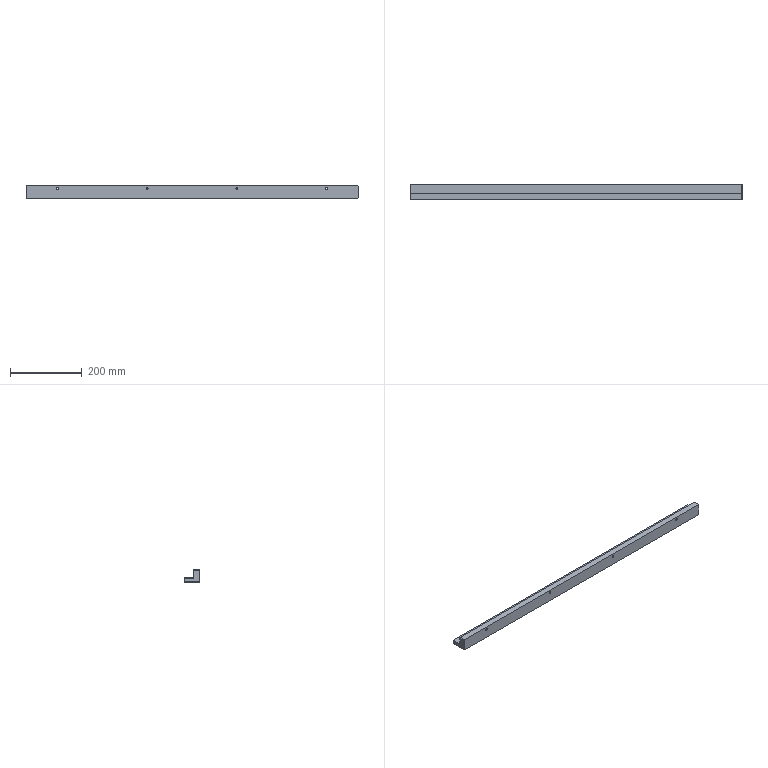Part | NX | features BREP 1 | 1 solid | 54 faces | box 926 x 44 x 35 mm | volume 847450 mm3 | cylinder 26 | plane 18 | cone 10 | commonest cylinder face diameters 3.3 x10 5.5 x8 10 x8
STEP:
#1=CARTESIAN_POINT('',(-463.,17.,16.5));
#2=VERTEX_POINT('',#1);
#3=CARTESIAN_POINT('',(-462.,17.,17.5));
#4=VERTEX_POINT('',#3);
#5=CARTESIAN_POINT('',(-462.,17.,17.5));
#6=DIRECTION('',(0.7071,0.,0.7071));
#7=VECTOR('',#6,1000.);
#8=LINE('',#5,#7);
#9=EDGE_CURVE('',#2,#4,#8,.T.);
#10=ORIENTED_EDGE('',*,*,#9,.F.);
#11=CARTESIAN_POINT('',(-463.,0.,16.5));
#12=VERTEX_POINT('',#11);
#13=CARTESIAN_POINT('',(-463.,44.,16.5));
#14=DIRECTION('',(0.,1.,0.));
#15=VECTOR('',#14,1000.);
#16=LINE('',#13,#15);
#17=EDGE_CURVE('',#12,#2,#16,.T.);
#18=ORIENTED_EDGE('',*,*,#17,.F.);
#19=CARTESIAN_POINT('',(-462.,0.,17.5));
#20=VERTEX_POINT('',#19);
#21=CARTESIAN_POINT('',(-462.,0.,17.5));
#22=DIRECTION('',(-0.7071,0.,-0.7071));
#23=VECTOR('',#22,1000.);
#24=LINE('',#21,#23);
#25=EDGE_CURVE('',#20,#12,#24,.T.);
#26=ORIENTED_EDGE('',*,*,#25,.F.);
#27=CARTESIAN_POINT('',(-462.,44.,17.5));
#28=DIRECTION('',(0.,-1.,0.));
#29=VECTOR('',#28,1000.);
#30=LINE('',#27,#29);
#31=EDGE_CURVE('',#4,#20,#30,.T.);
#32=ORIENTED_EDGE('',*,*,#31,.F.);
#33=EDGE_LOOP('',(#10,#18,#26,#32));
#34=FACE_BOUND('',#33,.T.);
#35=CARTESIAN_POINT('',(-462.,44.,17.5));
#36=DIRECTION('',(0.7071,0.,-0.7071));
#37=DIRECTION('',(0.,-1.,0.));
#38=AXIS2_PLACEMENT_3D('',#35,#36,#37);
#39=PLANE('',#38);
#40=ADVANCED_FACE('',(#34),#39,.F.);
#41=CARTESIAN_POINT('',(-463.,44.,-6.5));
#42=VERTEX_POINT('',#41);
#43=CARTESIAN_POINT('',(-462.,44.,-5.5));
#44=VERTEX_POINT('',#43);
#45=CARTESIAN_POINT('',(-228.25,44.,228.25));
#46=DIRECTION('',(0.7071,0.,0.7071));
#47=VECTOR('',#46,1000.);
#48=LINE('',#45,#47);
#49=EDGE_CURVE('',#42,#44,#48,.T.);
#50=ORIENTED_EDGE('',*,*,#49,.F.);
#51=CARTESIAN_POINT('',(-463.,17.,-6.5));
#52=VERTEX_POINT('',#51);
#53=CARTESIAN_POINT('',(-463.,44.,-6.5));
#54=DIRECTION('',(0.,1.,0.));
#55=VECTOR('',#54,1000.);
#56=LINE('',#53,#55);
#57=EDGE_CURVE('',#52,#42,#56,.T.);
#58=ORIENTED_EDGE('',*,*,#57,.F.);
#59=CARTESIAN_POINT('',(-462.,17.,-5.5));
#60=VERTEX_POINT('',#59);
#61=CARTESIAN_POINT('',(12.,17.,468.5));
#62=DIRECTION('',(-0.7071,0.,-0.7071));
#63=VECTOR('',#62,1000.);
#64=LINE('',#61,#63);
#65=EDGE_CURVE('',#60,#52,#64,.T.);
#66=ORIENTED_EDGE('',*,*,#65,.F.);
#67=CARTESIAN_POINT('',(-462.,44.,-5.5));
#68=DIRECTION('',(0.,-1.,0.));
#69=VECTOR('',#68,1000.);
#70=LINE('',#67,#69);
#71=EDGE_CURVE('',#44,#60,#70,.T.);
#72=ORIENTED_EDGE('',*,*,#71,.F.);
#73=EDGE_LOOP('',(#50,#58,#66,#72));
#74=FACE_BOUND('',#73,.T.);
#75=CARTESIAN_POINT('',(-462.,44.,-5.5));
#76=DIRECTION('',(0.7071,0.,-0.7071));
#77=DIRECTION('',(0.,-1.,0.));
#78=AXIS2_PLACEMENT_3D('',#75,#76,#77);
#79=PLANE('',#78);
#80=ADVANCED_FACE('',(#74),#79,.F.);
#81=CARTESIAN_POINT('',(-462.,44.,-17.5));
#82=VERTEX_POINT('',#81);
#83=CARTESIAN_POINT('',(-463.,44.,-16.5));
#84=VERTEX_POINT('',#83);
#85=CARTESIAN_POINT('',(-239.75,44.,-239.75));
#86=DIRECTION('',(-0.7071,0.,0.7071));
#87=VECTOR('',#86,1000.);
#88=LINE('',#85,#87);
#89=EDGE_CURVE('',#82,#84,#88,.T.);
#90=ORIENTED_EDGE('',*,*,#89,.F.);
#91=CARTESIAN_POINT('',(-462.,0.,-17.5));
#92=VERTEX_POINT('',#91);
#93=CARTESIAN_POINT('',(-462.,44.,-17.5));
#94=DIRECTION('',(0.,1.,0.));
#95=VECTOR('',#94,1000.);
#96=LINE('',#93,#95);
#97=EDGE_CURVE('',#92,#82,#96,.T.);
#98=ORIENTED_EDGE('',*,*,#97,.F.);
#99=CARTESIAN_POINT('',(-463.,0.,-16.5));
#100=VERTEX_POINT('',#99);
#101=CARTESIAN_POINT('',(-463.,0.,-16.5));
#102=DIRECTION('',(0.7071,0.,-0.7071));
#103=VECTOR('',#102,1000.);
#104=LINE('',#101,#103);
#105=EDGE_CURVE('',#100,#92,#104,.T.);
#106=ORIENTED_EDGE('',*,*,#105,.F.);
#107=CARTESIAN_POINT('',(-463.,44.,-16.5));
#108=DIRECTION('',(0.,-1.,0.));
#109=VECTOR('',#108,1000.);
#110=LINE('',#107,#109);
#111=EDGE_CURVE('',#84,#100,#110,.T.);
#112=ORIENTED_EDGE('',*,*,#111,.F.);
#113=EDGE_LOOP('',(#90,#98,#106,#112));
#114=FACE_BOUND('',#113,.T.);
#115=CARTESIAN_POINT('',(-463.,44.,-16.5));
#116=DIRECTION('',(0.7071,0.,0.7071));
#117=DIRECTION('',(0.,-1.,0.));
#118=AXIS2_PLACEMENT_3D('',#115,#116,#117);
#119=PLANE('',#118);
#120=ADVANCED_FACE('',(#114),#119,.F.);
#121=CARTESIAN_POINT('',(462.,44.,-5.5));
#122=VERTEX_POINT('',#121);
#123=CARTESIAN_POINT('',(463.,44.,-6.5));
#124=VERTEX_POINT('',#123);
#125=CARTESIAN_POINT('',(228.25,44.,228.25));
#126=DIRECTION('',(0.7071,0.,-0.7071));
#127=VECTOR('',#126,1000.);
#128=LINE('',#125,#127);
#129=EDGE_CURVE('',#122,#124,#128,.T.);
#130=ORIENTED_EDGE('',*,*,#129,.F.);
#131=CARTESIAN_POINT('',(462.,17.,-5.5));
#132=VERTEX_POINT('',#131);
#133=CARTESIAN_POINT('',(462.,44.,-5.5));
#134=DIRECTION('',(0.,1.,0.));
#135=VECTOR('',#134,1000.);
#136=LINE('',#133,#135);
#137=EDGE_CURVE('',#132,#122,#136,.T.);
#138=ORIENTED_EDGE('',*,*,#137,.F.);
#139=CARTESIAN_POINT('',(463.,17.,-6.5));
#140=VERTEX_POINT('',#139);
#141=CARTESIAN_POINT('',(451.,17.,5.5));
#142=DIRECTION('',(-0.7071,0.,0.7071));
#143=VECTOR('',#142,1000.);
#144=LINE('',#141,#143);
#145=EDGE_CURVE('',#140,#132,#144,.T.);
#146=ORIENTED_EDGE('',*,*,#145,.F.);
#147=CARTESIAN_POINT('',(463.,44.,-6.5));
#148=DIRECTION('',(0.,-1.,0.));
#149=VECTOR('',#148,1000.);
#150=LINE('',#147,#149);
#151=EDGE_CURVE('',#124,#140,#150,.T.);
#152=ORIENTED_EDGE('',*,*,#151,.F.);
#153=EDGE_LOOP('',(#130,#138,#146,#152));
#154=FACE_BOUND('',#153,.T.);
#155=CARTESIAN_POINT('',(463.,44.,-6.5));
#156=DIRECTION('',(-0.7071,0.,-0.7071));
#157=DIRECTION('',(0.,-1.,0.));
#158=AXIS2_PLACEMENT_3D('',#155,#156,#157);
#159=PLANE('',#158);
#160=ADVANCED_FACE('',(#154),#159,.F.);
#161=CARTESIAN_POINT('',(463.,44.,-16.5));
#162=VERTEX_POINT('',#161);
#163=CARTESIAN_POINT('',(462.,44.,-17.5));
#164=VERTEX_POINT('',#163);
#165=CARTESIAN_POINT('',(239.75,44.,-239.75));
#166=DIRECTION('',(-0.7071,0.,-0.7071));
#167=VECTOR('',#166,1000.);
#168=LINE('',#165,#167);
#169=EDGE_CURVE('',#162,#164,#168,.T.);
#170=ORIENTED_EDGE('',*,*,#169,.F.);
#171=CARTESIAN_POINT('',(463.,0.,-16.5));
#172=VERTEX_POINT('',#171);
#173=CARTESIAN_POINT('',(463.,44.,-16.5));
#174=DIRECTION('',(0.,1.,0.));
#175=VECTOR('',#174,1000.);
#176=LINE('',#173,#175);
#177=EDGE_CURVE('',#172,#162,#176,.T.);
#178=ORIENTED_EDGE('',*,*,#177,.F.);
#179=CARTESIAN_POINT('',(462.,0.,-17.5));
#180=VERTEX_POINT('',#179);
#181=CARTESIAN_POINT('',(462.,0.,-17.5));
#182=DIRECTION('',(0.7071,0.,0.7071));
#183=VECTOR('',#182,1000.);
#184=LINE('',#181,#183);
#185=EDGE_CURVE('',#180,#172,#184,.T.);
#186=ORIENTED_EDGE('',*,*,#185,.F.);
#187=CARTESIAN_POINT('',(462.,44.,-17.5));
#188=DIRECTION('',(0.,-1.,0.));
#189=VECTOR('',#188,1000.);
#190=LINE('',#187,#189);
#191=EDGE_CURVE('',#164,#180,#190,.T.);
#192=ORIENTED_EDGE('',*,*,#191,.F.);
#193=EDGE_LOOP('',(#170,#178,#186,#192));
#194=FACE_BOUND('',#193,.T.);
#195=CARTESIAN_POINT('',(462.,44.,-17.5));
#196=DIRECTION('',(-0.7071,0.,0.7071));
#197=DIRECTION('',(0.,-1.,0.));
#198=AXIS2_PLACEMENT_3D('',#195,#196,#197);
#199=PLANE('',#198);
#200=ADVANCED_FACE('',(#194),#199,.F.);
#201=CARTESIAN_POINT('',(462.,17.,17.5));
#202=VERTEX_POINT('',#201);
#203=CARTESIAN_POINT('',(463.,17.,16.5));
#204=VERTEX_POINT('',#203);
#205=CARTESIAN_POINT('',(463.,17.,16.5));
#206=DIRECTION('',(0.7071,0.,-0.7071));
#207=VECTOR('',#206,1000.);
#208=LINE('',#205,#207);
#209=EDGE_CURVE('',#202,#204,#208,.T.);
#210=ORIENTED_EDGE('',*,*,#209,.F.);
#211=CARTESIAN_POINT('',(462.,0.,17.5));
#212=VERTEX_POINT('',#211);
#213=CARTESIAN_POINT('',(462.,44.,17.5));
#214=DIRECTION('',(0.,1.,0.));
#215=VECTOR('',#214,1000.);
#216=LINE('',#213,#215);
#217=EDGE_CURVE('',#212,#202,#216,.T.);
#218=ORIENTED_EDGE('',*,*,#217,.F.);
#219=CARTESIAN_POINT('',(463.,0.,16.5));
#220=VERTEX_POINT('',#219);
#221=CARTESIAN_POINT('',(463.,0.,16.5));
#222=DIRECTION('',(-0.7071,0.,0.7071));
#223=VECTOR('',#222,1000.);
#224=LINE('',#221,#223);
#225=EDGE_CURVE('',#220,#212,#224,.T.);
#226=ORIENTED_EDGE('',*,*,#225,.F.);
#227=CARTESIAN_POINT('',(463.,44.,16.5));
#228=DIRECTION('',(0.,-1.,0.));
#229=VECTOR('',#228,1000.);
#230=LINE('',#227,#229);
#231=EDGE_CURVE('',#204,#220,#230,.T.);
#232=ORIENTED_EDGE('',*,*,#231,.F.);
#233=EDGE_LOOP('',(#210,#218,#226,#232));
#234=FACE_BOUND('',#233,.T.);
#235=CARTESIAN_POINT('',(463.,44.,16.5));
#236=DIRECTION('',(-0.7071,0.,-0.7071));
#237=DIRECTION('',(0.,-1.,0.));
#238=AXIS2_PLACEMENT_3D('',#235,#236,#237);
#239=PLANE('',#238);
#240=ADVANCED_FACE('',(#234),#239,.F.);
#241=CARTESIAN_POINT('',(-375.,17.,4.5));
#242=VERTEX_POINT('',#241);
#243=CARTESIAN_POINT('',(-375.,11.3,4.5));
#244=VERTEX_POINT('',#243);
#245=CARTESIAN_POINT('',(-375.,17.,4.5));
#246=DIRECTION('',(0.,1.,0.));
#247=VECTOR('',#246,1000.);
#248=LINE('',#245,#247);
#249=EDGE_CURVE('',#242,#244,#248,.F.);
#250=ORIENTED_EDGE('',*,*,#249,.T.);
#251=CARTESIAN_POINT('',(-375.,11.3,14.5));
#252=VERTEX_POINT('',#251);
#253=CARTESIAN_POINT('',(-375.,11.3,9.5));
#254=DIRECTION('',(0.,1.,0.));
#255=DIRECTION('',(0.,0.,1.));
#256=AXIS2_PLACEMENT_3D('',#253,#254,#255);
#257=CIRCLE('',#256,5.);
#258=EDGE_CURVE('',#252,#244,#257,.T.);
#259=ORIENTED_EDGE('',*,*,#258,.F.);
#260=CARTESIAN_POINT('',(-375.,17.,14.5));
#261=VERTEX_POINT('',#260);
#262=CARTESIAN_POINT('',(-375.,17.,14.5));
#263=DIRECTION('',(0.,1.,0.));
#264=VECTOR('',#263,1000.);
#265=LINE('',#262,#264);
#266=EDGE_CURVE('',#261,#252,#265,.F.);
#267=ORIENTED_EDGE('',*,*,#266,.F.);
#268=CARTESIAN_POINT('',(-375.,17.,9.5));
#269=DIRECTION('',(0.,1.,0.));
#270=DIRECTION('',(0.,0.,1.));
#271=AXIS2_PLACEMENT_3D('',#268,#269,#270);
#272=CIRCLE('',#271,5.);
#273=EDGE_CURVE('',#261,#242,#272,.T.);
#274=ORIENTED_EDGE('',*,*,#273,.T.);
#275=EDGE_LOOP('',(#250,#259,#267,#274));
#276=FACE_BOUND('',#275,.T.);
#277=CARTESIAN_POINT('',(-375.,17.,9.5));
#278=DIRECTION('',(0.,1.,0.));
#279=DIRECTION('',(0.,0.,1.));
#280=AXIS2_PLACEMENT_3D('',#277,#278,#279);
#281=CYLINDRICAL_SURFACE('',#280,5.);
#282=ADVANCED_FACE('',(#276),#281,.F.);
#283=ORIENTED_EDGE('',*,*,#258,.T.);
#284=CARTESIAN_POINT('',(-375.,11.3,9.5));
#285=DIRECTION('',(0.,1.,0.));
#286=DIRECTION('',(0.,0.,1.));
#287=AXIS2_PLACEMENT_3D('',#284,#285,#286);
#288=CIRCLE('',#287,5.);
#289=EDGE_CURVE('',#244,#252,#288,.T.);
#290=ORIENTED_EDGE('',*,*,#289,.T.);
#291=EDGE_LOOP('',(#283,#290));
#292=FACE_BOUND('',#291,.T.);
#293=CARTESIAN_POINT('',(-375.,11.3,12.25));
#294=VERTEX_POINT('',#293);
#295=CARTESIAN_POINT('',(-375.,11.3,6.75));
#296=VERTEX_POINT('',#295);
#297=CARTESIAN_POINT('',(-375.,11.3,9.5));
#298=DIRECTION('',(0.,1.,0.));
#299=DIRECTION('',(0.,0.,1.));
#300=AXIS2_PLACEMENT_3D('',#297,#298,#299);
#301=CIRCLE('',#300,2.75);
#302=EDGE_CURVE('',#294,#296,#301,.T.);
#303=ORIENTED_EDGE('',*,*,#302,.F.);
#304=CARTESIAN_POINT('',(-375.,11.3,9.5));
#305=DIRECTION('',(0.,1.,0.));
#306=DIRECTION('',(0.,0.,1.));
#307=AXIS2_PLACEMENT_3D('',#304,#305,#306);
#308=CIRCLE('',#307,2.75);
#309=EDGE_CURVE('',#296,#294,#308,.T.);
#310=ORIENTED_EDGE('',*,*,#309,.F.);
#311=EDGE_LOOP('',(#303,#310));
#312=FACE_BOUND('',#311,.T.);
#313=CARTESIAN_POINT('',(-372.25,11.3,9.5));
#314=DIRECTION('',(0.,-1.,0.));
#315=DIRECTION('',(0.,0.,-1.));
#316=AXIS2_PLACEMENT_3D('',#313,#314,#315);
#317=PLANE('',#316);
#318=ADVANCED_FACE('',(#292,#312),#317,.F.);
#319=CARTESIAN_POINT('',(-375.,0.,6.75));
#320=VERTEX_POINT('',#319);
#321=CARTESIAN_POINT('',(-375.,17.,6.75));
#322=DIRECTION('',(0.,1.,0.));
#323=VECTOR('',#322,1000.);
#324=LINE('',#321,#323);
#325=EDGE_CURVE('',#296,#320,#324,.F.);
#326=ORIENTED_EDGE('',*,*,#325,.T.);
#327=CARTESIAN_POINT('',(-375.,0.,12.25));
#328=VERTEX_POINT('',#327);
#329=CARTESIAN_POINT('',(-375.,0.,9.5));
#330=DIRECTION('',(0.,1.,0.));
#331=DIRECTION('',(0.,0.,1.));
#332=AXIS2_PLACEMENT_3D('',#329,#330,#331);
#333=CIRCLE('',#332,2.75);
#334=EDGE_CURVE('',#328,#320,#333,.T.);
#335=ORIENTED_EDGE('',*,*,#334,.F.);
#336=CARTESIAN_POINT('',(-375.,17.,12.25));
#337=DIRECTION('',(0.,1.,0.));
#338=VECTOR('',#337,1000.);
#339=LINE('',#336,#338);
#340=EDGE_CURVE('',#294,#328,#339,.F.);
#341=ORIENTED_EDGE('',*,*,#340,.F.);
#342=ORIENTED_EDGE('',*,*,#302,.T.);
#343=EDGE_LOOP('',(#326,#335,#341,#342));
#344=FACE_BOUND('',#343,.T.);
#345=CARTESIAN_POINT('',(-375.,17.,9.5));
#346=DIRECTION('',(0.,1.,0.));
#347=DIRECTION('',(0.,0.,1.));
#348=AXIS2_PLACEMENT_3D('',#345,#346,#347);
#349=CYLINDRICAL_SURFACE('',#348,2.75);
#350=ADVANCED_FACE('',(#344),#349,.F.);
#351=CARTESIAN_POINT('',(-125.,17.,4.5));
#352=VERTEX_POINT('',#351);
#353=CARTESIAN_POINT('',(-125.,11.3,4.5));
#354=VERTEX_POINT('',#353);
#355=CARTESIAN_POINT('',(-125.,17.,4.5));
#356=DIRECTION('',(0.,1.,0.));
#357=VECTOR('',#356,1000.);
#358=LINE('',#355,#357);
#359=EDGE_CURVE('',#352,#354,#358,.F.);
#360=ORIENTED_EDGE('',*,*,#359,.T.);
#361=CARTESIAN_POINT('',(-125.,11.3,14.5));
#362=VERTEX_POINT('',#361);
#363=CARTESIAN_POINT('',(-125.,11.3,9.5));
#364=DIRECTION('',(0.,1.,0.));
#365=DIRECTION('',(0.,0.,1.));
#366=AXIS2_PLACEMENT_3D('',#363,#364,#365);
#367=CIRCLE('',#366,5.);
#368=EDGE_CURVE('',#362,#354,#367,.T.);
#369=ORIENTED_EDGE('',*,*,#368,.F.);
#370=CARTESIAN_POINT('',(-125.,17.,14.5));
#371=VERTEX_POINT('',#370);
#372=CARTESIAN_POINT('',(-125.,17.,14.5));
#373=DIRECTION('',(0.,1.,0.));
#374=VECTOR('',#373,1000.);
#375=LINE('',#372,#374);
#376=EDGE_CURVE('',#371,#362,#375,.F.);
#377=ORIENTED_EDGE('',*,*,#376,.F.);
#378=CARTESIAN_POINT('',(-125.,17.,9.5));
#379=DIRECTION('',(0.,1.,0.));
#380=DIRECTION('',(0.,0.,1.));
#381=AXIS2_PLACEMENT_3D('',#378,#379,#380);
#382=CIRCLE('',#381,5.);
#383=EDGE_CURVE('',#371,#352,#382,.T.);
#384=ORIENTED_EDGE('',*,*,#383,.T.);
#385=EDGE_LOOP('',(#360,#369,#377,#384));
#386=FACE_BOUND('',#385,.T.);
#387=CARTESIAN_POINT('',(-125.,17.,9.5));
#388=DIRECTION('',(0.,1.,0.));
#389=DIRECTION('',(0.,0.,1.));
#390=AXIS2_PLACEMENT_3D('',#387,#388,#389);
#391=CYLINDRICAL_SURFACE('',#390,5.);
#392=ADVANCED_FACE('',(#386),#391,.F.);
#393=ORIENTED_EDGE('',*,*,#368,.T.);
#394=CARTESIAN_POINT('',(-125.,11.3,9.5));
#395=DIRECTION('',(0.,1.,0.));
#396=DIRECTION('',(0.,0.,1.));
#397=AXIS2_PLACEMENT_3D('',#394,#395,#396);
#398=CIRCLE('',#397,5.);
#399=EDGE_CURVE('',#354,#362,#398,.T.);
#400=ORIENTED_EDGE('',*,*,#399,.T.);
#401=EDGE_LOOP('',(#393,#400));
#402=FACE_BOUND('',#401,.T.);
#403=CARTESIAN_POINT('',(-125.,11.3,12.25));
#404=VERTEX_POINT('',#403);
#405=CARTESIAN_POINT('',(-125.,11.3,6.75));
#406=VERTEX_POINT('',#405);
#407=CARTESIAN_POINT('',(-125.,11.3,9.5));
#408=DIRECTION('',(0.,1.,0.));
#409=DIRECTION('',(0.,0.,1.));
#410=AXIS2_PLACEMENT_3D('',#407,#408,#409);
#411=CIRCLE('',#410,2.75);
#412=EDGE_CURVE('',#404,#406,#411,.T.);
#413=ORIENTED_EDGE('',*,*,#412,.F.);
#414=CARTESIAN_POINT('',(-125.,11.3,9.5));
#415=DIRECTION('',(0.,1.,0.));
#416=DIRECTION('',(0.,0.,1.));
#417=AXIS2_PLACEMENT_3D('',#414,#415,#416);
#418=CIRCLE('',#417,2.75);
#419=EDGE_CURVE('',#406,#404,#418,.T.);
#420=ORIENTED_EDGE('',*,*,#419,.F.);
#421=EDGE_LOOP('',(#413,#420));
#422=FACE_BOUND('',#421,.T.);
#423=CARTESIAN_POINT('',(-122.25,11.3,9.5));
#424=DIRECTION('',(0.,-1.,0.));
#425=DIRECTION('',(0.,0.,-1.));
#426=AXIS2_PLACEMENT_3D('',#423,#424,#425);
#427=PLANE('',#426);
#428=ADVANCED_FACE('',(#402,#422),#427,.F.);
#429=CARTESIAN_POINT('',(-125.,0.,6.75));
#430=VERTEX_POINT('',#429);
#431=CARTESIAN_POINT('',(-125.,17.,6.75));
#432=DIRECTION('',(0.,1.,0.));
#433=VECTOR('',#432,1000.);
#434=LINE('',#431,#433);
#435=EDGE_CURVE('',#406,#430,#434,.F.);
#436=ORIENTED_EDGE('',*,*,#435,.T.);
#437=CARTESIAN_POINT('',(-125.,0.,12.25));
#438=VERTEX_POINT('',#437);
#439=CARTESIAN_POINT('',(-125.,0.,9.5));
#440=DIRECTION('',(0.,1.,0.));
#441=DIRECTION('',(0.,0.,1.));
#442=AXIS2_PLACEMENT_3D('',#439,#440,#441);
#443=CIRCLE('',#442,2.75);
#444=EDGE_CURVE('',#438,#430,#443,.T.);
#445=ORIENTED_EDGE('',*,*,#444,.F.);
#446=CARTESIAN_POINT('',(-125.,17.,12.25));
#447=DIRECTION('',(0.,1.,0.));
#448=VECTOR('',#447,1000.);
#449=LINE('',#446,#448);
#450=EDGE_CURVE('',#404,#438,#449,.F.);
#451=ORIENTED_EDGE('',*,*,#450,.F.);
#452=ORIENTED_EDGE('',*,*,#412,.T.);
#453=EDGE_LOOP('',(#436,#445,#451,#452));
#454=FACE_BOUND('',#453,.T.);
#455=CARTESIAN_POINT('',(-125.,17.,9.5));
#456=DIRECTION('',(0.,1.,0.));
#457=DIRECTION('',(0.,0.,1.));
#458=AXIS2_PLACEMENT_3D('',#455,#456,#457);
#459=CYLINDRICAL_SURFACE('',#458,2.75);
#460=ADVANCED_FACE('',(#454),#459,.F.);
#461=CARTESIAN_POINT('',(125.,17.,4.5));
#462=VERTEX_POINT('',#461);
#463=CARTESIAN_POINT('',(125.,11.3,4.5));
#464=VERTEX_POINT('',#463);
#465=CARTESIAN_POINT('',(125.,17.,4.5));
#466=DIRECTION('',(0.,1.,0.));
#467=VECTOR('',#466,1000.);
#468=LINE('',#465,#467);
#469=EDGE_CURVE('',#462,#464,#468,.F.);
#470=ORIENTED_EDGE('',*,*,#469,.T.);
#471=CARTESIAN_POINT('',(125.,11.3,14.5));
#472=VERTEX_POINT('',#471);
#473=CARTESIAN_POINT('',(125.,11.3,9.5));
#474=DIRECTION('',(0.,1.,0.));
#475=DIRECTION('',(0.,0.,1.));
#476=AXIS2_PLACEMENT_3D('',#473,#474,#475);
#477=CIRCLE('',#476,5.);
#478=EDGE_CURVE('',#472,#464,#477,.T.);
#479=ORIENTED_EDGE('',*,*,#478,.F.);
#480=CARTESIAN_POINT('',(125.,17.,14.5));
#481=VERTEX_POINT('',#480);
#482=CARTESIAN_POINT('',(125.,17.,14.5));
#483=DIRECTION('',(0.,1.,0.));
#484=VECTOR('',#483,1000.);
#485=LINE('',#482,#484);
#486=EDGE_CURVE('',#481,#472,#485,.F.);
#487=ORIENTED_EDGE('',*,*,#486,.F.);
#488=CARTESIAN_POINT('',(125.,17.,9.5));
#489=DIRECTION('',(0.,1.,0.));
#490=DIRECTION('',(0.,0.,1.));
#491=AXIS2_PLACEMENT_3D('',#488,#489,#490);
#492=CIRCLE('',#491,5.);
#493=EDGE_CURVE('',#481,#462,#492,.T.);
#494=ORIENTED_EDGE('',*,*,#493,.T.);
#495=EDGE_LOOP('',(#470,#479,#487,#494));
#496=FACE_BOUND('',#495,.T.);
#497=CARTESIAN_POINT('',(125.,17.,9.5));
#498=DIRECTION('',(0.,1.,0.));
#499=DIRECTION('',(0.,0.,1.));
#500=AXIS2_PLACEMENT_3D('',#497,#498,#499);
#501=CYLINDRICAL_SURFACE('',#500,5.);
#502=ADVANCED_FACE('',(#496),#501,.F.);
#503=ORIENTED_EDGE('',*,*,#478,.T.);
#504=CARTESIAN_POINT('',(125.,11.3,9.5));
#505=DIRECTION('',(0.,1.,0.));
#506=DIRECTION('',(0.,0.,1.));
#507=AXIS2_PLACEMENT_3D('',#504,#505,#506);
#508=CIRCLE('',#507,5.);
#509=EDGE_CURVE('',#464,#472,#508,.T.);
#510=ORIENTED_EDGE('',*,*,#509,.T.);
#511=EDGE_LOOP('',(#503,#510));
#512=FACE_BOUND('',#511,.T.);
#513=CARTESIAN_POINT('',(125.,11.3,12.25));
#514=VERTEX_POINT('',#513);
#515=CARTESIAN_POINT('',(125.,11.3,6.75));
#516=VERTEX_POINT('',#515);
#517=CARTESIAN_POINT('',(125.,11.3,9.5));
#518=DIRECTION('',(0.,1.,0.));
#519=DIRECTION('',(0.,0.,1.));
#520=AXIS2_PLACEMENT_3D('',#517,#518,#519);
#521=CIRCLE('',#520,2.75);
#522=EDGE_CURVE('',#514,#516,#521,.T.);
#523=ORIENTED_EDGE('',*,*,#522,.F.);
#524=CARTESIAN_POINT('',(125.,11.3,9.5));
#525=DIRECTION('',(0.,1.,0.));
#526=DIRECTION('',(0.,0.,1.));
#527=AXIS2_PLACEMENT_3D('',#524,#525,#526);
#528=CIRCLE('',#527,2.75);
#529=EDGE_CURVE('',#516,#514,#528,.T.);
#530=ORIENTED_EDGE('',*,*,#529,.F.);
#531=EDGE_LOOP('',(#523,#530));
#532=FACE_BOUND('',#531,.T.);
#533=CARTESIAN_POINT('',(127.75,11.3,9.5));
#534=DIRECTION('',(0.,-1.,0.));
#535=DIRECTION('',(0.,0.,-1.));
#536=AXIS2_PLACEMENT_3D('',#533,#534,#535);
#537=PLANE('',#536);
#538=ADVANCED_FACE('',(#512,#532),#537,.F.);
#539=CARTESIAN_POINT('',(125.,0.,6.75));
#540=VERTEX_POINT('',#539);
#541=CARTESIAN_POINT('',(125.,17.,6.75));
#542=DIRECTION('',(0.,1.,0.));
#543=VECTOR('',#542,1000.);
#544=LINE('',#541,#543);
#545=EDGE_CURVE('',#516,#540,#544,.F.);
#546=ORIENTED_EDGE('',*,*,#545,.T.);
#547=CARTESIAN_POINT('',(125.,0.,12.25));
#548=VERTEX_POINT('',#547);
#549=CARTESIAN_POINT('',(125.,0.,9.5));
#550=DIRECTION('',(0.,1.,0.));
#551=DIRECTION('',(0.,0.,1.));
#552=AXIS2_PLACEMENT_3D('',#549,#550,#551);
#553=CIRCLE('',#552,2.75);
#554=EDGE_CURVE('',#548,#540,#553,.T.);
#555=ORIENTED_EDGE('',*,*,#554,.F.);
#556=CARTESIAN_POINT('',(125.,17.,12.25));
#557=DIRECTION('',(0.,1.,0.));
#558=VECTOR('',#557,1000.);
#559=LINE('',#556,#558);
#560=EDGE_CURVE('',#514,#548,#559,.F.);
#561=ORIENTED_EDGE('',*,*,#560,.F.);
#562=ORIENTED_EDGE('',*,*,#522,.T.);
#563=EDGE_LOOP('',(#546,#555,#561,#562));
#564=FACE_BOUND('',#563,.T.);
#565=CARTESIAN_POINT('',(125.,17.,9.5));
#566=DIRECTION('',(0.,1.,0.));
#567=DIRECTION('',(0.,0.,1.));
#568=AXIS2_PLACEMENT_3D('',#565,#566,#567);
#569=CYLINDRICAL_SURFACE('',#568,2.75);
#570=ADVANCED_FACE('',(#564),#569,.F.);
#571=CARTESIAN_POINT('',(375.,17.,4.5));
#572=VERTEX_POINT('',#571);
#573=CARTESIAN_POINT('',(375.,11.3,4.5));
#574=VERTEX_POINT('',#573);
#575=CARTESIAN_POINT('',(375.,17.,4.5));
#576=DIRECTION('',(0.,1.,0.));
#577=VECTOR('',#576,1000.);
#578=LINE('',#575,#577);
#579=EDGE_CURVE('',#572,#574,#578,.F.);
#580=ORIENTED_EDGE('',*,*,#579,.T.);
#581=CARTESIAN_POINT('',(375.,11.3,14.5));
#582=VERTEX_POINT('',#581);
#583=CARTESIAN_POINT('',(375.,11.3,9.5));
#584=DIRECTION('',(0.,1.,0.));
#585=DIRECTION('',(0.,0.,1.));
#586=AXIS2_PLACEMENT_3D('',#583,#584,#585);
#587=CIRCLE('',#586,5.);
#588=EDGE_CURVE('',#582,#574,#587,.T.);
#589=ORIENTED_EDGE('',*,*,#588,.F.);
#590=CARTESIAN_POINT('',(375.,17.,14.5));
#591=VERTEX_POINT('',#590);
#592=CARTESIAN_POINT('',(375.,17.,14.5));
#593=DIRECTION('',(0.,1.,0.));
#594=VECTOR('',#593,1000.);
#595=LINE('',#592,#594);
#596=EDGE_CURVE('',#591,#582,#595,.F.);
#597=ORIENTED_EDGE('',*,*,#596,.F.);
#598=CARTESIAN_POINT('',(375.,17.,9.5));
#599=DIRECTION('',(0.,1.,0.));
#600=DIRECTION('',(0.,0.,1.));
#601=AXIS2_PLACEMENT_3D('',#598,#599,#600);
#602=CIRCLE('',#601,5.);
#603=EDGE_CURVE('',#591,#572,#602,.T.);
#604=ORIENTED_EDGE('',*,*,#603,.T.);
#605=EDGE_LOOP('',(#580,#589,#597,#604));
#606=FACE_BOUND('',#605,.T.);
#607=CARTESIAN_POINT('',(375.,17.,9.5));
#608=DIRECTION('',(0.,1.,0.));
#609=DIRECTION('',(0.,0.,1.));
#610=AXIS2_PLACEMENT_3D('',#607,#608,#609);
#611=CYLINDRICAL_SURFACE('',#610,5.);
#612=ADVANCED_FACE('',(#606),#611,.F.);
#613=ORIENTED_EDGE('',*,*,#588,.T.);
#614=CARTESIAN_POINT('',(375.,11.3,9.5));
#615=DIRECTION('',(0.,1.,0.));
#616=DIRECTION('',(0.,0.,1.));
#617=AXIS2_PLACEMENT_3D('',#614,#615,#616);
#618=CIRCLE('',#617,5.);
#619=EDGE_CURVE('',#574,#582,#618,.T.);
#620=ORIENTED_EDGE('',*,*,#619,.T.);
#621=EDGE_LOOP('',(#613,#620));
#622=FACE_BOUND('',#621,.T.);
#623=CARTESIAN_POINT('',(375.,11.3,12.25));
#624=VERTEX_POINT('',#623);
#625=CARTESIAN_POINT('',(375.,11.3,6.75));
#626=VERTEX_POINT('',#625);
#627=CARTESIAN_POINT('',(375.,11.3,9.5));
#628=DIRECTION('',(0.,1.,0.));
#629=DIRECTION('',(0.,0.,1.));
#630=AXIS2_PLACEMENT_3D('',#627,#628,#629);
#631=CIRCLE('',#630,2.75);
#632=EDGE_CURVE('',#624,#626,#631,.T.);
#633=ORIENTED_EDGE('',*,*,#632,.F.);
#634=CARTESIAN_POINT('',(375.,11.3,9.5));
#635=DIRECTION('',(0.,1.,0.));
#636=DIRECTION('',(0.,0.,1.));
#637=AXIS2_PLACEMENT_3D('',#634,#635,#636);
#638=CIRCLE('',#637,2.75);
#639=EDGE_CURVE('',#626,#624,#638,.T.);
#640=ORIENTED_EDGE('',*,*,#639,.F.);
#641=EDGE_LOOP('',(#633,#640));
#642=FACE_BOUND('',#641,.T.);
#643=CARTESIAN_POINT('',(377.75,11.3,9.5));
#644=DIRECTION('',(0.,-1.,0.));
#645=DIRECTION('',(0.,0.,-1.));
#646=AXIS2_PLACEMENT_3D('',#643,#644,#645);
#647=PLANE('',#646);
#648=ADVANCED_FACE('',(#622,#642),#647,.F.);
#649=CARTESIAN_POINT('',(375.,0.,6.75));
#650=VERTEX_POINT('',#649);
#651=CARTESIAN_POINT('',(375.,17.,6.75));
#652=DIRECTION('',(0.,1.,0.));
#653=VECTOR('',#652,1000.);
#654=LINE('',#651,#653);
#655=EDGE_CURVE('',#626,#650,#654,.F.);
#656=ORIENTED_EDGE('',*,*,#655,.T.);
#657=CARTESIAN_POINT('',(375.,0.,12.25));
#658=VERTEX_POINT('',#657);
#659=CARTESIAN_POINT('',(375.,0.,9.5));
#660=DIRECTION('',(0.,1.,0.));
#661=DIRECTION('',(0.,0.,1.));
#662=AXIS2_PLACEMENT_3D('',#659,#660,#661);
#663=CIRCLE('',#662,2.75);
#664=EDGE_CURVE('',#658,#650,#663,.T.);
#665=ORIENTED_EDGE('',*,*,#664,.F.);
#666=CARTESIAN_POINT('',(375.,17.,12.25));
#667=DIRECTION('',(0.,1.,0.));
#668=VECTOR('',#667,1000.);
#669=LINE('',#666,#668);
#670=EDGE_CURVE('',#624,#658,#669,.F.);
#671=ORIENTED_EDGE('',*,*,#670,.F.);
#672=ORIENTED_EDGE('',*,*,#632,.T.);
#673=EDGE_LOOP('',(#656,#665,#671,#672));
#674=FACE_BOUND('',#673,.T.);
#675=CARTESIAN_POINT('',(375.,17.,9.5));
#676=DIRECTION('',(0.,1.,0.));
#677=DIRECTION('',(0.,0.,1.));
#678=AXIS2_PLACEMENT_3D('',#675,#676,#677);
#679=CYLINDRICAL_SURFACE('',#678,2.75);
#680=ADVANCED_FACE('',(#674),#679,.F.);
#681=CARTESIAN_POINT('',(-440.,44.,-13.15));
#682=VERTEX_POINT('',#681);
#683=CARTESIAN_POINT('',(-440.,30.5,-13.15));
#684=VERTEX_POINT('',#683);
#685=CARTESIAN_POINT('',(-440.,44.,-13.15));
#686=DIRECTION('',(0.,1.,0.));
#687=VECTOR('',#686,1000.);
#688=LINE('',#685,#687);
#689=EDGE_CURVE('',#682,#684,#688,.F.);
#690=ORIENTED_EDGE('',*,*,#689,.T.);
#691=CARTESIAN_POINT('',(-440.,30.5,-9.85));
#692=VERTEX_POINT('',#691);
#693=CARTESIAN_POINT('',(-440.,30.5,-11.5));
#694=DIRECTION('',(0.,1.,0.));
#695=DIRECTION('',(0.,0.,1.));
#696=AXIS2_PLACEMENT_3D('',#693,#694,#695);
#697=CIRCLE('',#696,1.65);
#698=EDGE_CURVE('',#692,#684,#697,.T.);
#699=ORIENTED_EDGE('',*,*,#698,.F.);
#700=CARTESIAN_POINT('',(-440.,44.,-9.85));
#701=VERTEX_POINT('',#700);
#702=CARTESIAN_POINT('',(-440.,44.,-9.85));
#703=DIRECTION('',(0.,1.,0.));
#704=VECTOR('',#703,1000.);
#705=LINE('',#702,#704);
#706=EDGE_CURVE('',#701,#692,#705,.F.);
#707=ORIENTED_EDGE('',*,*,#706,.F.);
#708=CARTESIAN_POINT('',(-440.,44.,-11.5));
#709=DIRECTION('',(0.,1.,0.));
#710=DIRECTION('',(0.,0.,1.));
#711=AXIS2_PLACEMENT_3D('',#708,#709,#710);
#712=CIRCLE('',#711,1.65);
#713=EDGE_CURVE('',#701,#682,#712,.T.);
#714=ORIENTED_EDGE('',*,*,#713,.T.);
#715=EDGE_LOOP('',(#690,#699,#707,#714));
#716=FACE_BOUND('',#715,.T.);
#717=CARTESIAN_POINT('',(-440.,44.,-11.5));
#718=DIRECTION('',(0.,1.,0.));
#719=DIRECTION('',(0.,0.,1.));
#720=AXIS2_PLACEMENT_3D('',#717,#718,#719);
#721=CYLINDRICAL_SURFACE('',#720,1.65);
#722=ADVANCED_FACE('',(#716),#721,.F.);
#723=CARTESIAN_POINT('',(-440.,29.509,-11.5));
#724=VERTEX_POINT('',#723);
#725=CARTESIAN_POINT('',(-440.,30.5,-13.15));
#726=DIRECTION('',(0.,0.515,-0.8572));
#727=VECTOR('',#726,1000.);
#728=LINE('',#725,#727);
#729=EDGE_CURVE('',#724,#684,#728,.T.);
#730=ORIENTED_EDGE('',*,*,#729,.F.);
#731=CARTESIAN_POINT('',(-440.,30.5,-9.85));
#732=DIRECTION('',(0.,0.515,0.8572));
#733=VECTOR('',#732,1000.);
#734=LINE('',#731,#733);
#735=EDGE_CURVE('',#724,#692,#734,.T.);
#736=ORIENTED_EDGE('',*,*,#735,.T.);
#737=ORIENTED_EDGE('',*,*,#698,.T.);
#738=EDGE_LOOP('',(#730,#736,#737));
#739=FACE_BOUND('',#738,.T.);
#740=CARTESIAN_POINT('',(-440.,30.5,-11.5));
#741=DIRECTION('',(0.,1.,0.));
#742=DIRECTION('',(0.,0.,1.));
#743=AXIS2_PLACEMENT_3D('',#740,#741,#742);
#744=CONICAL_SURFACE('',#743,1.65,1.03);
#745=ADVANCED_FACE('',(#739),#744,.F.);
#746=CARTESIAN_POINT('',(-220.,44.,-13.15));
#747=VERTEX_POINT('',#746);
#748=CARTESIAN_POINT('',(-220.,30.5,-13.15));
#749=VERTEX_POINT('',#748);
#750=CARTESIAN_POINT('',(-220.,44.,-13.15));
#751=DIRECTION('',(0.,1.,0.));
#752=VECTOR('',#751,1000.);
#753=LINE('',#750,#752);
#754=EDGE_CURVE('',#747,#749,#753,.F.);
#755=ORIENTED_EDGE('',*,*,#754,.T.);
#756=CARTESIAN_POINT('',(-220.,30.5,-9.85));
#757=VERTEX_POINT('',#756);
#758=CARTESIAN_POINT('',(-220.,30.5,-11.5));
#759=DIRECTION('',(0.,1.,0.));
#760=DIRECTION('',(0.,0.,1.));
#761=AXIS2_PLACEMENT_3D('',#758,#759,#760);
#762=CIRCLE('',#761,1.65);
#763=EDGE_CURVE('',#757,#749,#762,.T.);
#764=ORIENTED_EDGE('',*,*,#763,.F.);
#765=CARTESIAN_POINT('',(-220.,44.,-9.85));
#766=VERTEX_POINT('',#765);
#767=CARTESIAN_POINT('',(-220.,44.,-9.85));
#768=DIRECTION('',(0.,1.,0.));
#769=VECTOR('',#768,1000.);
#770=LINE('',#767,#769);
#771=EDGE_CURVE('',#766,#757,#770,.F.);
#772=ORIENTED_EDGE('',*,*,#771,.F.);
#773=CARTESIAN_POINT('',(-220.,44.,-11.5));
#774=DIRECTION('',(0.,1.,0.));
#775=DIRECTION('',(0.,0.,1.));
#776=AXIS2_PLACEMENT_3D('',#773,#774,#775);
#777=CIRCLE('',#776,1.65);
#778=EDGE_CURVE('',#766,#747,#777,.T.);
#779=ORIENTED_EDGE('',*,*,#778,.T.);
#780=EDGE_LOOP('',(#755,#764,#772,#779));
#781=FACE_BOUND('',#780,.T.);
#782=CARTESIAN_POINT('',(-220.,44.,-11.5));
#783=DIRECTION('',(0.,1.,0.));
#784=DIRECTION('',(0.,0.,1.));
#785=AXIS2_PLACEMENT_3D('',#782,#783,#784);
#786=CYLINDRICAL_SURFACE('',#785,1.65);
#787=ADVANCED_FACE('',(#781),#786,.F.);
#788=CARTESIAN_POINT('',(-220.,29.509,-11.5));
#789=VERTEX_POINT('',#788);
#790=CARTESIAN_POINT('',(-220.,30.5,-13.15));
#791=DIRECTION('',(0.,0.515,-0.8572));
#792=VECTOR('',#791,1000.);
#793=LINE('',#790,#792);
#794=EDGE_CURVE('',#789,#749,#793,.T.);
#795=ORIENTED_EDGE('',*,*,#794,.F.);
#796=CARTESIAN_POINT('',(-220.,30.5,-9.85));
#797=DIRECTION('',(0.,0.515,0.8572));
#798=VECTOR('',#797,1000.);
#799=LINE('',#796,#798);
#800=EDGE_CURVE('',#789,#757,#799,.T.);
#801=ORIENTED_EDGE('',*,*,#800,.T.);
#802=ORIENTED_EDGE('',*,*,#763,.T.);
#803=EDGE_LOOP('',(#795,#801,#802));
#804=FACE_BOUND('',#803,.T.);
#805=CARTESIAN_POINT('',(-220.,30.5,-11.5));
#806=DIRECTION('',(0.,1.,0.));
#807=DIRECTION('',(0.,0.,1.));
#808=AXIS2_PLACEMENT_3D('',#805,#806,#807);
#809=CONICAL_SURFACE('',#808,1.65,1.03);
#810=ADVANCED_FACE('',(#804),#809,.F.);
#811=CARTESIAN_POINT('',(0.,44.,-13.15));
#812=VERTEX_POINT('',#811);
#813=CARTESIAN_POINT('',(0.,30.5,-13.15));
#814=VERTEX_POINT('',#813);
#815=CARTESIAN_POINT('',(0.,44.,-13.15));
#816=DIRECTION('',(0.,1.,0.));
#817=VECTOR('',#816,1000.);
#818=LINE('',#815,#817);
#819=EDGE_CURVE('',#812,#814,#818,.F.);
#820=ORIENTED_EDGE('',*,*,#819,.T.);
#821=CARTESIAN_POINT('',(0.,30.5,-9.85));
#822=VERTEX_POINT('',#821);
#823=CARTESIAN_POINT('',(0.,30.5,-11.5));
#824=DIRECTION('',(0.,1.,0.));
#825=DIRECTION('',(0.,0.,1.));
#826=AXIS2_PLACEMENT_3D('',#823,#824,#825);
#827=CIRCLE('',#826,1.65);
#828=EDGE_CURVE('',#822,#814,#827,.T.);
#829=ORIENTED_EDGE('',*,*,#828,.F.);
#830=CARTESIAN_POINT('',(0.,44.,-9.85));
#831=VERTEX_POINT('',#830);
#832=CARTESIAN_POINT('',(0.,44.,-9.85));
#833=DIRECTION('',(0.,1.,0.));
#834=VECTOR('',#833,1000.);
#835=LINE('',#832,#834);
#836=EDGE_CURVE('',#831,#822,#835,.F.);
#837=ORIENTED_EDGE('',*,*,#836,.F.);
#838=CARTESIAN_POINT('',(0.,44.,-11.5));
#839=DIRECTION('',(0.,1.,0.));
#840=DIRECTION('',(0.,0.,1.));
#841=AXIS2_PLACEMENT_3D('',#838,#839,#840);
#842=CIRCLE('',#841,1.65);
#843=EDGE_CURVE('',#831,#812,#842,.T.);
#844=ORIENTED_EDGE('',*,*,#843,.T.);
#845=EDGE_LOOP('',(#820,#829,#837,#844));
#846=FACE_BOUND('',#845,.T.);
#847=CARTESIAN_POINT('',(0.,44.,-11.5));
#848=DIRECTION('',(0.,1.,0.));
#849=DIRECTION('',(0.,0.,1.));
#850=AXIS2_PLACEMENT_3D('',#847,#848,#849);
#851=CYLINDRICAL_SURFACE('',#850,1.65);
#852=ADVANCED_FACE('',(#846),#851,.F.);
#853=CARTESIAN_POINT('',(0.,29.509,-11.5));
#854=VERTEX_POINT('',#853);
#855=CARTESIAN_POINT('',(0.,30.5,-13.15));
#856=DIRECTION('',(0.,0.515,-0.8572));
#857=VECTOR('',#856,1000.);
#858=LINE('',#855,#857);
#859=EDGE_CURVE('',#854,#814,#858,.T.);
#860=ORIENTED_EDGE('',*,*,#859,.F.);
#861=CARTESIAN_POINT('',(0.,30.5,-9.85));
#862=DIRECTION('',(0.,0.515,0.8572));
#863=VECTOR('',#862,1000.);
#864=LINE('',#861,#863);
#865=EDGE_CURVE('',#854,#822,#864,.T.);
#866=ORIENTED_EDGE('',*,*,#865,.T.);
#867=ORIENTED_EDGE('',*,*,#828,.T.);
#868=EDGE_LOOP('',(#860,#866,#867));
#869=FACE_BOUND('',#868,.T.);
#870=CARTESIAN_POINT('',(0.,30.5,-11.5));
#871=DIRECTION('',(0.,1.,0.));
#872=DIRECTION('',(0.,0.,1.));
#873=AXIS2_PLACEMENT_3D('',#870,#871,#872);
#874=CONICAL_SURFACE('',#873,1.65,1.03);
#875=ADVANCED_FACE('',(#869),#874,.F.);
#876=CARTESIAN_POINT('',(220.,44.,-13.15));
#877=VERTEX_POINT('',#876);
#878=CARTESIAN_POINT('',(220.,30.5,-13.15));
#879=VERTEX_POINT('',#878);
#880=CARTESIAN_POINT('',(220.,44.,-13.15));
#881=DIRECTION('',(0.,1.,0.));
#882=VECTOR('',#881,1000.);
#883=LINE('',#880,#882);
#884=EDGE_CURVE('',#877,#879,#883,.F.);
#885=ORIENTED_EDGE('',*,*,#884,.T.);
#886=CARTESIAN_POINT('',(220.,30.5,-9.85));
#887=VERTEX_POINT('',#886);
#888=CARTESIAN_POINT('',(220.,30.5,-11.5));
#889=DIRECTION('',(0.,1.,0.));
#890=DIRECTION('',(0.,0.,1.));
#891=AXIS2_PLACEMENT_3D('',#888,#889,#890);
#892=CIRCLE('',#891,1.65);
#893=EDGE_CURVE('',#887,#879,#892,.T.);
#894=ORIENTED_EDGE('',*,*,#893,.F.);
#895=CARTESIAN_POINT('',(220.,44.,-9.85));
#896=VERTEX_POINT('',#895);
#897=CARTESIAN_POINT('',(220.,44.,-9.85));
#898=DIRECTION('',(0.,1.,0.));
#899=VECTOR('',#898,1000.);
#900=LINE('',#897,#899);
#901=EDGE_CURVE('',#896,#887,#900,.F.);
#902=ORIENTED_EDGE('',*,*,#901,.F.);
#903=CARTESIAN_POINT('',(220.,44.,-11.5));
#904=DIRECTION('',(0.,1.,0.));
#905=DIRECTION('',(0.,0.,1.));
#906=AXIS2_PLACEMENT_3D('',#903,#904,#905);
#907=CIRCLE('',#906,1.65);
#908=EDGE_CURVE('',#896,#877,#907,.T.);
#909=ORIENTED_EDGE('',*,*,#908,.T.);
#910=EDGE_LOOP('',(#885,#894,#902,#909));
#911=FACE_BOUND('',#910,.T.);
#912=CARTESIAN_POINT('',(220.,44.,-11.5));
#913=DIRECTION('',(0.,1.,0.));
#914=DIRECTION('',(0.,0.,1.));
#915=AXIS2_PLACEMENT_3D('',#912,#913,#914);
#916=CYLINDRICAL_SURFACE('',#915,1.65);
#917=ADVANCED_FACE('',(#911),#916,.F.);
#918=CARTESIAN_POINT('',(220.,29.509,-11.5));
#919=VERTEX_POINT('',#918);
#920=CARTESIAN_POINT('',(220.,30.5,-13.15));
#921=DIRECTION('',(0.,0.515,-0.8572));
#922=VECTOR('',#921,1000.);
#923=LINE('',#920,#922);
#924=EDGE_CURVE('',#919,#879,#923,.T.);
#925=ORIENTED_EDGE('',*,*,#924,.F.);
#926=CARTESIAN_POINT('',(220.,30.5,-9.85));
#927=DIRECTION('',(0.,0.515,0.8572));
#928=VECTOR('',#927,1000.);
#929=LINE('',#926,#928);
#930=EDGE_CURVE('',#919,#887,#929,.T.);
#931=ORIENTED_EDGE('',*,*,#930,.T.);
#932=ORIENTED_EDGE('',*,*,#893,.T.);
#933=EDGE_LOOP('',(#925,#931,#932));
#934=FACE_BOUND('',#933,.T.);
#935=CARTESIAN_POINT('',(220.,30.5,-11.5));
#936=DIRECTION('',(0.,1.,0.));
#937=DIRECTION('',(0.,0.,1.));
#938=AXIS2_PLACEMENT_3D('',#935,#936,#937);
#939=CONICAL_SURFACE('',#938,1.65,1.03);
#940=ADVANCED_FACE('',(#934),#939,.F.);
#941=CARTESIAN_POINT('',(440.,44.,-13.15));
#942=VERTEX_POINT('',#941);
#943=CARTESIAN_POINT('',(440.,30.5,-13.15));
#944=VERTEX_POINT('',#943);
#945=CARTESIAN_POINT('',(440.,44.,-13.15));
#946=DIRECTION('',(0.,1.,0.));
#947=VECTOR('',#946,1000.);
#948=LINE('',#945,#947);
#949=EDGE_CURVE('',#942,#944,#948,.F.);
#950=ORIENTED_EDGE('',*,*,#949,.T.);
#951=CARTESIAN_POINT('',(440.,30.5,-9.85));
#952=VERTEX_POINT('',#951);
#953=CARTESIAN_POINT('',(440.,30.5,-11.5));
#954=DIRECTION('',(0.,1.,0.));
#955=DIRECTION('',(0.,0.,1.));
#956=AXIS2_PLACEMENT_3D('',#953,#954,#955);
#957=CIRCLE('',#956,1.65);
#958=EDGE_CURVE('',#952,#944,#957,.T.);
#959=ORIENTED_EDGE('',*,*,#958,.F.);
#960=CARTESIAN_POINT('',(440.,44.,-9.85));
#961=VERTEX_POINT('',#960);
#962=CARTESIAN_POINT('',(440.,44.,-9.85));
#963=DIRECTION('',(0.,1.,0.));
#964=VECTOR('',#963,1000.);
#965=LINE('',#962,#964);
#966=EDGE_CURVE('',#961,#952,#965,.F.);
#967=ORIENTED_EDGE('',*,*,#966,.F.);
#968=CARTESIAN_POINT('',(440.,44.,-11.5));
#969=DIRECTION('',(0.,1.,0.));
#970=DIRECTION('',(0.,0.,1.));
#971=AXIS2_PLACEMENT_3D('',#968,#969,#970);
#972=CIRCLE('',#971,1.65);
#973=EDGE_CURVE('',#961,#942,#972,.T.);
#974=ORIENTED_EDGE('',*,*,#973,.T.);
#975=EDGE_LOOP('',(#950,#959,#967,#974));
#976=FACE_BOUND('',#975,.T.);
#977=CARTESIAN_POINT('',(440.,44.,-11.5));
#978=DIRECTION('',(0.,1.,0.));
#979=DIRECTION('',(0.,0.,1.));
#980=AXIS2_PLACEMENT_3D('',#977,#978,#979);
#981=CYLINDRICAL_SURFACE('',#980,1.65);
#982=ADVANCED_FACE('',(#976),#981,.F.);
#983=CARTESIAN_POINT('',(440.,29.509,-11.5));
#984=VERTEX_POINT('',#983);
#985=CARTESIAN_POINT('',(440.,30.5,-13.15));
#986=DIRECTION('',(0.,0.515,-0.8572));
#987=VECTOR('',#986,1000.);
#988=LINE('',#985,#987);
#989=EDGE_CURVE('',#984,#944,#988,.T.);
#990=ORIENTED_EDGE('',*,*,#989,.F.);
#991=CARTESIAN_POINT('',(440.,30.5,-9.85));
#992=DIRECTION('',(0.,0.515,0.8572));
#993=VECTOR('',#992,1000.);
#994=LINE('',#991,#993);
#995=EDGE_CURVE('',#984,#952,#994,.T.);
#996=ORIENTED_EDGE('',*,*,#995,.T.);
#997=ORIENTED_EDGE('',*,*,#958,.T.);
#998=EDGE_LOOP('',(#990,#996,#997));
#999=FACE_BOUND('',#998,.T.);
#1000=CARTESIAN_POINT('',(440.,30.5,-11.5));
#1001=DIRECTION('',(0.,1.,0.));
#1002=DIRECTION('',(0.,0.,1.));
#1003=AXIS2_PLACEMENT_3D('',#1000,#1001,#1002);
#1004=CONICAL_SURFACE('',#1003,1.65,1.03);
#1005=ADVANCED_FACE('',(#999),#1004,.F.);
#1006=CARTESIAN_POINT('',(463.,17.,-5.5));
#1007=DIRECTION('',(-1.,0.,0.));
#1008=VECTOR('',#1007,1000.);
#1009=LINE('',#1006,#1008);
#1010=EDGE_CURVE('',#132,#60,#1009,.T.);
#1011=ORIENTED_EDGE('',*,*,#1010,.F.);
#1012=ORIENTED_EDGE('',*,*,#137,.T.);
#1013=CARTESIAN_POINT('',(463.,44.,-5.5));
#1014=DIRECTION('',(-1.,0.,0.));
#1015=VECTOR('',#1014,1000.);
#1016=LINE('',#1013,#1015);
#1017=EDGE_CURVE('',#122,#44,#1016,.T.);
#1018=ORIENTED_EDGE('',*,*,#1017,.T.);
#1019=ORIENTED_EDGE('',*,*,#71,.T.);
#1020=EDGE_LOOP('',(#1011,#1012,#1018,#1019));
#1021=FACE_BOUND('',#1020,.T.);
#1022=CARTESIAN_POINT('',(463.,44.,-5.5));
#1023=DIRECTION('',(0.,0.,-1.));
#1024=DIRECTION('',(0.,1.,0.));
#1025=AXIS2_PLACEMENT_3D('',#1022,#1023,#1024);
#1026=PLANE('',#1025);
#1027=ADVANCED_FACE('',(#1021),#1026,.F.);
#1028=CARTESIAN_POINT('',(463.,17.,17.5));
#1029=DIRECTION('',(-1.,0.,0.));
#1030=VECTOR('',#1029,1000.);
#1031=LINE('',#1028,#1030);
#1032=EDGE_CURVE('',#202,#4,#1031,.T.);
#1033=ORIENTED_EDGE('',*,*,#1032,.F.);
#1034=ORIENTED_EDGE('',*,*,#209,.T.);
#1035=CARTESIAN_POINT('',(463.,17.,17.5));
#1036=DIRECTION('',(0.,0.,1.));
#1037=VECTOR('',#1036,1000.);
#1038=LINE('',#1035,#1037);
#1039=EDGE_CURVE('',#140,#204,#1038,.T.);
#1040=ORIENTED_EDGE('',*,*,#1039,.F.);
#1041=ORIENTED_EDGE('',*,*,#145,.T.);
#1042=ORIENTED_EDGE('',*,*,#1010,.T.);
#1043=ORIENTED_EDGE('',*,*,#65,.T.);
#1044=CARTESIAN_POINT('',(-463.,17.,17.5));
#1045=DIRECTION('',(0.,0.,1.));
#1046=VECTOR('',#1045,1000.);
#1047=LINE('',#1044,#1046);
#1048=EDGE_CURVE('',#52,#2,#1047,.T.);
#1049=ORIENTED_EDGE('',*,*,#1048,.T.);
#1050=ORIENTED_EDGE('',*,*,#9,.T.);
#1051=EDGE_LOOP('',(#1033,#1034,#1040,#1041,#1042,#1043,#1049,#1050));
#1052=FACE_BOUND('',#1051,.T.);
#1053=ORIENTED_EDGE('',*,*,#603,.F.);
#1054=CARTESIAN_POINT('',(375.,17.,9.5));
#1055=DIRECTION('',(0.,1.,0.));
#1056=DIRECTION('',(0.,0.,1.));
#1057=AXIS2_PLACEMENT_3D('',#1054,#1055,#1056);
#1058=CIRCLE('',#1057,5.);
#1059=EDGE_CURVE('',#572,#591,#1058,.T.);
#1060=ORIENTED_EDGE('',*,*,#1059,.F.);
#1061=EDGE_LOOP('',(#1053,#1060));
#1062=FACE_BOUND('',#1061,.T.);
#1063=ORIENTED_EDGE('',*,*,#493,.F.);
#1064=CARTESIAN_POINT('',(125.,17.,9.5));
#1065=DIRECTION('',(0.,1.,0.));
#1066=DIRECTION('',(0.,0.,1.));
#1067=AXIS2_PLACEMENT_3D('',#1064,#1065,#1066);
#1068=CIRCLE('',#1067,5.);
#1069=EDGE_CURVE('',#462,#481,#1068,.T.);
#1070=ORIENTED_EDGE('',*,*,#1069,.F.);
#1071=EDGE_LOOP('',(#1063,#1070));
#1072=FACE_BOUND('',#1071,.T.);
#1073=ORIENTED_EDGE('',*,*,#383,.F.);
#1074=CARTESIAN_POINT('',(-125.,17.,9.5));
#1075=DIRECTION('',(0.,1.,0.));
#1076=DIRECTION('',(0.,0.,1.));
#1077=AXIS2_PLACEMENT_3D('',#1074,#1075,#1076);
#1078=CIRCLE('',#1077,5.);
#1079=EDGE_CURVE('',#352,#371,#1078,.T.);
#1080=ORIENTED_EDGE('',*,*,#1079,.F.);
#1081=EDGE_LOOP('',(#1073,#1080));
#1082=FACE_BOUND('',#1081,.T.);
#1083=ORIENTED_EDGE('',*,*,#273,.F.);
#1084=CARTESIAN_POINT('',(-375.,17.,9.5));
#1085=DIRECTION('',(0.,1.,0.));
#1086=DIRECTION('',(0.,0.,1.));
#1087=AXIS2_PLACEMENT_3D('',#1084,#1085,#1086);
#1088=CIRCLE('',#1087,5.);
#1089=EDGE_CURVE('',#242,#261,#1088,.T.);
#1090=ORIENTED_EDGE('',*,*,#1089,.F.);
#1091=EDGE_LOOP('',(#1083,#1090));
#1092=FACE_BOUND('',#1091,.T.);
#1093=CARTESIAN_POINT('',(463.,17.,17.5));
#1094=DIRECTION('',(0.,-1.,0.));
#1095=DIRECTION('',(0.,0.,-1.));
#1096=AXIS2_PLACEMENT_3D('',#1093,#1094,#1095);
#1097=PLANE('',#1096);
#1098=ADVANCED_FACE('',(#1052,#1062,#1072,#1082,#1092),#1097,.F.);
#1099=CARTESIAN_POINT('',(463.,0.,17.5));
#1100=DIRECTION('',(0.,0.,-1.));
#1101=VECTOR('',#1100,1000.);
#1102=LINE('',#1099,#1101);
#1103=EDGE_CURVE('',#220,#172,#1102,.T.);
#1104=ORIENTED_EDGE('',*,*,#1103,.F.);
#1105=ORIENTED_EDGE('',*,*,#225,.T.);
#1106=CARTESIAN_POINT('',(463.,0.,17.5));
#1107=DIRECTION('',(1.,0.,0.));
#1108=VECTOR('',#1107,1000.);
#1109=LINE('',#1106,#1108);
#1110=EDGE_CURVE('',#20,#212,#1109,.T.);
#1111=ORIENTED_EDGE('',*,*,#1110,.F.);
#1112=ORIENTED_EDGE('',*,*,#25,.T.);
#1113=CARTESIAN_POINT('',(-463.,0.,17.5));
#1114=DIRECTION('',(0.,0.,1.));
#1115=VECTOR('',#1114,1000.);
#1116=LINE('',#1113,#1115);
#1117=EDGE_CURVE('',#100,#12,#1116,.T.);
#1118=ORIENTED_EDGE('',*,*,#1117,.F.);
#1119=ORIENTED_EDGE('',*,*,#105,.T.);
#1120=CARTESIAN_POINT('',(463.,0.,-17.5));
#1121=DIRECTION('',(-1.,0.,0.));
#1122=VECTOR('',#1121,1000.);
#1123=LINE('',#1120,#1122);
#1124=EDGE_CURVE('',#180,#92,#1123,.T.);
#1125=ORIENTED_EDGE('',*,*,#1124,.F.);
#1126=ORIENTED_EDGE('',*,*,#185,.T.);
#1127=EDGE_LOOP('',(#1104,#1105,#1111,#1112,#1118,#1119,#1125,#1126));
#1128=FACE_BOUND('',#1127,.T.);
#1129=ORIENTED_EDGE('',*,*,#664,.T.);
#1130=CARTESIAN_POINT('',(375.,0.,9.5));
#1131=DIRECTION('',(0.,1.,0.));
#1132=DIRECTION('',(0.,0.,1.));
#1133=AXIS2_PLACEMENT_3D('',#1130,#1131,#1132);
#1134=CIRCLE('',#1133,2.75);
#1135=EDGE_CURVE('',#650,#658,#1134,.T.);
#1136=ORIENTED_EDGE('',*,*,#1135,.T.);
#1137=EDGE_LOOP('',(#1129,#1136));
#1138=FACE_BOUND('',#1137,.T.);
#1139=ORIENTED_EDGE('',*,*,#554,.T.);
#1140=CARTESIAN_POINT('',(125.,0.,9.5));
#1141=DIRECTION('',(0.,1.,0.));
#1142=DIRECTION('',(0.,0.,1.));
#1143=AXIS2_PLACEMENT_3D('',#1140,#1141,#1142);
#1144=CIRCLE('',#1143,2.75);
#1145=EDGE_CURVE('',#540,#548,#1144,.T.);
#1146=ORIENTED_EDGE('',*,*,#1145,.T.);
#1147=EDGE_LOOP('',(#1139,#1146));
#1148=FACE_BOUND('',#1147,.T.);
#1149=ORIENTED_EDGE('',*,*,#444,.T.);
#1150=CARTESIAN_POINT('',(-125.,0.,9.5));
#1151=DIRECTION('',(0.,1.,0.));
#1152=DIRECTION('',(0.,0.,1.));
#1153=AXIS2_PLACEMENT_3D('',#1150,#1151,#1152);
#1154=CIRCLE('',#1153,2.75);
#1155=EDGE_CURVE('',#430,#438,#1154,.T.);
#1156=ORIENTED_EDGE('',*,*,#1155,.T.);
#1157=EDGE_LOOP('',(#1149,#1156));
#1158=FACE_BOUND('',#1157,.T.);
#1159=ORIENTED_EDGE('',*,*,#334,.T.);
#1160=CARTESIAN_POINT('',(-375.,0.,9.5));
#1161=DIRECTION('',(0.,1.,0.));
#1162=DIRECTION('',(0.,0.,1.));
#1163=AXIS2_PLACEMENT_3D('',#1160,#1161,#1162);
#1164=CIRCLE('',#1163,2.75);
#1165=EDGE_CURVE('',#320,#328,#1164,.T.);
#1166=ORIENTED_EDGE('',*,*,#1165,.T.);
#1167=EDGE_LOOP('',(#1159,#1166));
#1168=FACE_BOUND('',#1167,.T.);
#1169=CARTESIAN_POINT('',(0.,0.,0.));
#1170=DIRECTION('',(0.,1.,0.));
#1171=DIRECTION('',(0.,0.,1.));
#1172=AXIS2_PLACEMENT_3D('',#1169,#1170,#1171);
#1173=PLANE('',#1172);
#1174=ADVANCED_FACE('',(#1128,#1138,#1148,#1158,#1168),#1173,.F.);
#1175=CARTESIAN_POINT('',(463.,44.,17.5));
#1176=DIRECTION('',(0.,0.,-1.));
#1177=VECTOR('',#1176,1000.);
#1178=LINE('',#1175,#1177);
#1179=EDGE_CURVE('',#124,#162,#1178,.T.);
#1180=ORIENTED_EDGE('',*,*,#1179,.T.);
#1181=ORIENTED_EDGE('',*,*,#169,.T.);
#1182=CARTESIAN_POINT('',(463.,44.,-17.5));
#1183=DIRECTION('',(-1.,0.,0.));
#1184=VECTOR('',#1183,1000.);
#1185=LINE('',#1182,#1184);
#1186=EDGE_CURVE('',#164,#82,#1185,.T.);
#1187=ORIENTED_EDGE('',*,*,#1186,.T.);
#1188=ORIENTED_EDGE('',*,*,#89,.T.);
#1189=CARTESIAN_POINT('',(-463.,44.,17.5));
#1190=DIRECTION('',(0.,0.,1.));
#1191=VECTOR('',#1190,1000.);
#1192=LINE('',#1189,#1191);
#1193=EDGE_CURVE('',#84,#42,#1192,.T.);
#1194=ORIENTED_EDGE('',*,*,#1193,.T.);
#1195=ORIENTED_EDGE('',*,*,#49,.T.);
#1196=ORIENTED_EDGE('',*,*,#1017,.F.);
#1197=ORIENTED_EDGE('',*,*,#129,.T.);
#1198=EDGE_LOOP('',(#1180,#1181,#1187,#1188,#1194,#1195,#1196,#1197));
#1199=FACE_BOUND('',#1198,.T.);
#1200=ORIENTED_EDGE('',*,*,#973,.F.);
#1201=CARTESIAN_POINT('',(440.,44.,-11.5));
#1202=DIRECTION('',(0.,1.,0.));
#1203=DIRECTION('',(0.,0.,1.));
#1204=AXIS2_PLACEMENT_3D('',#1201,#1202,#1203);
#1205=CIRCLE('',#1204,1.65);
#1206=EDGE_CURVE('',#942,#961,#1205,.T.);
#1207=ORIENTED_EDGE('',*,*,#1206,.F.);
#1208=EDGE_LOOP('',(#1200,#1207));
#1209=FACE_BOUND('',#1208,.T.);
#1210=ORIENTED_EDGE('',*,*,#908,.F.);
#1211=CARTESIAN_POINT('',(220.,44.,-11.5));
#1212=DIRECTION('',(0.,1.,0.));
#1213=DIRECTION('',(0.,0.,1.));
#1214=AXIS2_PLACEMENT_3D('',#1211,#1212,#1213);
#1215=CIRCLE('',#1214,1.65);
#1216=EDGE_CURVE('',#877,#896,#1215,.T.);
#1217=ORIENTED_EDGE('',*,*,#1216,.F.);
#1218=EDGE_LOOP('',(#1210,#1217));
#1219=FACE_BOUND('',#1218,.T.);
#1220=ORIENTED_EDGE('',*,*,#843,.F.);
#1221=CARTESIAN_POINT('',(0.,44.,-11.5));
#1222=DIRECTION('',(0.,1.,0.));
#1223=DIRECTION('',(0.,0.,1.));
#1224=AXIS2_PLACEMENT_3D('',#1221,#1222,#1223);
#1225=CIRCLE('',#1224,1.65);
#1226=EDGE_CURVE('',#812,#831,#1225,.T.);
#1227=ORIENTED_EDGE('',*,*,#1226,.F.);
#1228=EDGE_LOOP('',(#1220,#1227));
#1229=FACE_BOUND('',#1228,.T.);
#1230=ORIENTED_EDGE('',*,*,#778,.F.);
#1231=CARTESIAN_POINT('',(-220.,44.,-11.5));
#1232=DIRECTION('',(0.,1.,0.));
#1233=DIRECTION('',(0.,0.,1.));
#1234=AXIS2_PLACEMENT_3D('',#1231,#1232,#1233);
#1235=CIRCLE('',#1234,1.65);
#1236=EDGE_CURVE('',#747,#766,#1235,.T.);
#1237=ORIENTED_EDGE('',*,*,#1236,.F.);
#1238=EDGE_LOOP('',(#1230,#1237));
#1239=FACE_BOUND('',#1238,.T.);
#1240=ORIENTED_EDGE('',*,*,#713,.F.);
#1241=CARTESIAN_POINT('',(-440.,44.,-11.5));
#1242=DIRECTION('',(0.,1.,0.));
#1243=DIRECTION('',(0.,0.,1.));
#1244=AXIS2_PLACEMENT_3D('',#1241,#1242,#1243);
#1245=CIRCLE('',#1244,1.65);
#1246=EDGE_CURVE('',#682,#701,#1245,.T.);
#1247=ORIENTED_EDGE('',*,*,#1246,.F.);
#1248=EDGE_LOOP('',(#1240,#1247));
#1249=FACE_BOUND('',#1248,.T.);
#1250=CARTESIAN_POINT('',(0.,44.,0.));
#1251=DIRECTION('',(0.,1.,0.));
#1252=DIRECTION('',(0.,0.,1.));
#1253=AXIS2_PLACEMENT_3D('',#1250,#1251,#1252);
#1254=PLANE('',#1253);
#1255=ADVANCED_FACE('',(#1199,#1209,#1219,#1229,#1239,#1249),#1254,.T.);
#1256=ORIENTED_EDGE('',*,*,#1186,.F.);
#1257=ORIENTED_EDGE('',*,*,#191,.T.);
#1258=ORIENTED_EDGE('',*,*,#1124,.T.);
#1259=ORIENTED_EDGE('',*,*,#97,.T.);
#1260=EDGE_LOOP('',(#1256,#1257,#1258,#1259));
#1261=FACE_BOUND('',#1260,.T.);
#1262=CARTESIAN_POINT('',(463.,44.,-17.5));
#1263=DIRECTION('',(0.,0.,1.));
#1264=DIRECTION('',(1.,0.,0.));
#1265=AXIS2_PLACEMENT_3D('',#1262,#1263,#1264);
#1266=PLANE('',#1265);
#1267=ADVANCED_FACE('',(#1261),#1266,.F.);
#1268=ORIENTED_EDGE('',*,*,#1039,.T.);
#1269=ORIENTED_EDGE('',*,*,#231,.T.);
#1270=ORIENTED_EDGE('',*,*,#1103,.T.);
#1271=ORIENTED_EDGE('',*,*,#177,.T.);
#1272=ORIENTED_EDGE('',*,*,#1179,.F.);
#1273=ORIENTED_EDGE('',*,*,#151,.T.);
#1274=EDGE_LOOP('',(#1268,#1269,#1270,#1271,#1272,#1273));
#1275=FACE_BOUND('',#1274,.T.);
#1276=CARTESIAN_POINT('',(463.,44.,17.5));
#1277=DIRECTION('',(-1.,0.,0.));
#1278=DIRECTION('',(0.,0.,1.));
#1279=AXIS2_PLACEMENT_3D('',#1276,#1277,#1278);
#1280=PLANE('',#1279);
#1281=ADVANCED_FACE('',(#1275),#1280,.F.);
#1282=ORIENTED_EDGE('',*,*,#1110,.T.);
#1283=ORIENTED_EDGE('',*,*,#217,.T.);
#1284=ORIENTED_EDGE('',*,*,#1032,.T.);
#1285=ORIENTED_EDGE('',*,*,#31,.T.);
#1286=EDGE_LOOP('',(#1282,#1283,#1284,#1285));
#1287=FACE_BOUND('',#1286,.T.);
#1288=CARTESIAN_POINT('',(463.,44.,17.5));
#1289=DIRECTION('',(0.,0.,-1.));
#1290=DIRECTION('',(-1.,0.,0.));
#1291=AXIS2_PLACEMENT_3D('',#1288,#1289,#1290);
#1292=PLANE('',#1291);
#1293=ADVANCED_FACE('',(#1287),#1292,.F.);
#1294=ORIENTED_EDGE('',*,*,#1193,.F.);
#1295=ORIENTED_EDGE('',*,*,#111,.T.);
#1296=ORIENTED_EDGE('',*,*,#1117,.T.);
#1297=ORIENTED_EDGE('',*,*,#17,.T.);
#1298=ORIENTED_EDGE('',*,*,#1048,.F.);
#1299=ORIENTED_EDGE('',*,*,#57,.T.);
#1300=EDGE_LOOP('',(#1294,#1295,#1296,#1297,#1298,#1299));
#1301=FACE_BOUND('',#1300,.T.);
#1302=CARTESIAN_POINT('',(-463.,44.,17.5));
#1303=DIRECTION('',(1.,0.,0.));
#1304=DIRECTION('',(0.,0.,-1.));
#1305=AXIS2_PLACEMENT_3D('',#1302,#1303,#1304);
#1306=PLANE('',#1305);
#1307=ADVANCED_FACE('',(#1301),#1306,.F.);
#1308=ORIENTED_EDGE('',*,*,#995,.F.);
#1309=ORIENTED_EDGE('',*,*,#989,.T.);
#1310=CARTESIAN_POINT('',(440.,30.5,-11.5));
#1311=DIRECTION('',(0.,1.,0.));
#1312=DIRECTION('',(0.,0.,1.));
#1313=AXIS2_PLACEMENT_3D('',#1310,#1311,#1312);
#1314=CIRCLE('',#1313,1.65);
#1315=EDGE_CURVE('',#944,#952,#1314,.T.);
#1316=ORIENTED_EDGE('',*,*,#1315,.T.);
#1317=EDGE_LOOP('',(#1308,#1309,#1316));
#1318=FACE_BOUND('',#1317,.T.);
#1319=CARTESIAN_POINT('',(440.,30.5,-11.5));
#1320=DIRECTION('',(0.,1.,0.));
#1321=DIRECTION('',(0.,0.,1.));
#1322=AXIS2_PLACEMENT_3D('',#1319,#1320,#1321);
#1323=CONICAL_SURFACE('',#1322,1.65,1.03);
#1324=ADVANCED_FACE('',(#1318),#1323,.F.);
#1325=ORIENTED_EDGE('',*,*,#1315,.F.);
#1326=ORIENTED_EDGE('',*,*,#949,.F.);
#1327=ORIENTED_EDGE('',*,*,#1206,.T.);
#1328=ORIENTED_EDGE('',*,*,#966,.T.);
#1329=EDGE_LOOP('',(#1325,#1326,#1327,#1328));
#1330=FACE_BOUND('',#1329,.T.);
#1331=CARTESIAN_POINT('',(440.,44.,-11.5));
#1332=DIRECTION('',(0.,1.,0.));
#1333=DIRECTION('',(0.,0.,1.));
#1334=AXIS2_PLACEMENT_3D('',#1331,#1332,#1333);
#1335=CYLINDRICAL_SURFACE('',#1334,1.65);
#1336=ADVANCED_FACE('',(#1330),#1335,.F.);
#1337=ORIENTED_EDGE('',*,*,#930,.F.);
#1338=ORIENTED_EDGE('',*,*,#924,.T.);
#1339=CARTESIAN_POINT('',(220.,30.5,-11.5));
#1340=DIRECTION('',(0.,1.,0.));
#1341=DIRECTION('',(0.,0.,1.));
#1342=AXIS2_PLACEMENT_3D('',#1339,#1340,#1341);
#1343=CIRCLE('',#1342,1.65);
#1344=EDGE_CURVE('',#879,#887,#1343,.T.);
#1345=ORIENTED_EDGE('',*,*,#1344,.T.);
#1346=EDGE_LOOP('',(#1337,#1338,#1345));
#1347=FACE_BOUND('',#1346,.T.);
#1348=CARTESIAN_POINT('',(220.,30.5,-11.5));
#1349=DIRECTION('',(0.,1.,0.));
#1350=DIRECTION('',(0.,0.,1.));
#1351=AXIS2_PLACEMENT_3D('',#1348,#1349,#1350);
#1352=CONICAL_SURFACE('',#1351,1.65,1.03);
#1353=ADVANCED_FACE('',(#1347),#1352,.F.);
#1354=ORIENTED_EDGE('',*,*,#1344,.F.);
#1355=ORIENTED_EDGE('',*,*,#884,.F.);
#1356=ORIENTED_EDGE('',*,*,#1216,.T.);
#1357=ORIENTED_EDGE('',*,*,#901,.T.);
#1358=EDGE_LOOP('',(#1354,#1355,#1356,#1357));
#1359=FACE_BOUND('',#1358,.T.);
#1360=CARTESIAN_POINT('',(220.,44.,-11.5));
#1361=DIRECTION('',(0.,1.,0.));
#1362=DIRECTION('',(0.,0.,1.));
#1363=AXIS2_PLACEMENT_3D('',#1360,#1361,#1362);
#1364=CYLINDRICAL_SURFACE('',#1363,1.65);
#1365=ADVANCED_FACE('',(#1359),#1364,.F.);
#1366=ORIENTED_EDGE('',*,*,#865,.F.);
#1367=ORIENTED_EDGE('',*,*,#859,.T.);
#1368=CARTESIAN_POINT('',(0.,30.5,-11.5));
#1369=DIRECTION('',(0.,1.,0.));
#1370=DIRECTION('',(0.,0.,1.));
#1371=AXIS2_PLACEMENT_3D('',#1368,#1369,#1370);
#1372=CIRCLE('',#1371,1.65);
#1373=EDGE_CURVE('',#814,#822,#1372,.T.);
#1374=ORIENTED_EDGE('',*,*,#1373,.T.);
#1375=EDGE_LOOP('',(#1366,#1367,#1374));
#1376=FACE_BOUND('',#1375,.T.);
#1377=CARTESIAN_POINT('',(0.,30.5,-11.5));
#1378=DIRECTION('',(0.,1.,0.));
#1379=DIRECTION('',(0.,0.,1.));
#1380=AXIS2_PLACEMENT_3D('',#1377,#1378,#1379);
#1381=CONICAL_SURFACE('',#1380,1.65,1.03);
#1382=ADVANCED_FACE('',(#1376),#1381,.F.);
#1383=ORIENTED_EDGE('',*,*,#1373,.F.);
#1384=ORIENTED_EDGE('',*,*,#819,.F.);
#1385=ORIENTED_EDGE('',*,*,#1226,.T.);
#1386=ORIENTED_EDGE('',*,*,#836,.T.);
#1387=EDGE_LOOP('',(#1383,#1384,#1385,#1386));
#1388=FACE_BOUND('',#1387,.T.);
#1389=CARTESIAN_POINT('',(0.,44.,-11.5));
#1390=DIRECTION('',(0.,1.,0.));
#1391=DIRECTION('',(0.,0.,1.));
#1392=AXIS2_PLACEMENT_3D('',#1389,#1390,#1391);
#1393=CYLINDRICAL_SURFACE('',#1392,1.65);
#1394=ADVANCED_FACE('',(#1388),#1393,.F.);
#1395=ORIENTED_EDGE('',*,*,#800,.F.);
#1396=ORIENTED_EDGE('',*,*,#794,.T.);
#1397=CARTESIAN_POINT('',(-220.,30.5,-11.5));
#1398=DIRECTION('',(0.,1.,0.));
#1399=DIRECTION('',(0.,0.,1.));
#1400=AXIS2_PLACEMENT_3D('',#1397,#1398,#1399);
#1401=CIRCLE('',#1400,1.65);
#1402=EDGE_CURVE('',#749,#757,#1401,.T.);
#1403=ORIENTED_EDGE('',*,*,#1402,.T.);
#1404=EDGE_LOOP('',(#1395,#1396,#1403));
#1405=FACE_BOUND('',#1404,.T.);
#1406=CARTESIAN_POINT('',(-220.,30.5,-11.5));
#1407=DIRECTION('',(0.,1.,0.));
#1408=DIRECTION('',(0.,0.,1.));
#1409=AXIS2_PLACEMENT_3D('',#1406,#1407,#1408);
#1410=CONICAL_SURFACE('',#1409,1.65,1.03);
#1411=ADVANCED_FACE('',(#1405),#1410,.F.);
#1412=ORIENTED_EDGE('',*,*,#1402,.F.);
#1413=ORIENTED_EDGE('',*,*,#754,.F.);
#1414=ORIENTED_EDGE('',*,*,#1236,.T.);
#1415=ORIENTED_EDGE('',*,*,#771,.T.);
#1416=EDGE_LOOP('',(#1412,#1413,#1414,#1415));
#1417=FACE_BOUND('',#1416,.T.);
#1418=CARTESIAN_POINT('',(-220.,44.,-11.5));
#1419=DIRECTION('',(0.,1.,0.));
#1420=DIRECTION('',(0.,0.,1.));
#1421=AXIS2_PLACEMENT_3D('',#1418,#1419,#1420);
#1422=CYLINDRICAL_SURFACE('',#1421,1.65);
#1423=ADVANCED_FACE('',(#1417),#1422,.F.);
#1424=ORIENTED_EDGE('',*,*,#735,.F.);
#1425=ORIENTED_EDGE('',*,*,#729,.T.);
#1426=CARTESIAN_POINT('',(-440.,30.5,-11.5));
#1427=DIRECTION('',(0.,1.,0.));
#1428=DIRECTION('',(0.,0.,1.));
#1429=AXIS2_PLACEMENT_3D('',#1426,#1427,#1428);
#1430=CIRCLE('',#1429,1.65);
#1431=EDGE_CURVE('',#684,#692,#1430,.T.);
#1432=ORIENTED_EDGE('',*,*,#1431,.T.);
#1433=EDGE_LOOP('',(#1424,#1425,#1432));
#1434=FACE_BOUND('',#1433,.T.);
#1435=CARTESIAN_POINT('',(-440.,30.5,-11.5));
#1436=DIRECTION('',(0.,1.,0.));
#1437=DIRECTION('',(0.,0.,1.));
#1438=AXIS2_PLACEMENT_3D('',#1435,#1436,#1437);
#1439=CONICAL_SURFACE('',#1438,1.65,1.03);
#1440=ADVANCED_FACE('',(#1434),#1439,.F.);
#1441=ORIENTED_EDGE('',*,*,#1431,.F.);
#1442=ORIENTED_EDGE('',*,*,#689,.F.);
#1443=ORIENTED_EDGE('',*,*,#1246,.T.);
#1444=ORIENTED_EDGE('',*,*,#706,.T.);
#1445=EDGE_LOOP('',(#1441,#1442,#1443,#1444));
#1446=FACE_BOUND('',#1445,.T.);
#1447=CARTESIAN_POINT('',(-440.,44.,-11.5));
#1448=DIRECTION('',(0.,1.,0.));
#1449=DIRECTION('',(0.,0.,1.));
#1450=AXIS2_PLACEMENT_3D('',#1447,#1448,#1449);
#1451=CYLINDRICAL_SURFACE('',#1450,1.65);
#1452=ADVANCED_FACE('',(#1446),#1451,.F.);
#1453=ORIENTED_EDGE('',*,*,#1135,.F.);
#1454=ORIENTED_EDGE('',*,*,#655,.F.);
#1455=ORIENTED_EDGE('',*,*,#639,.T.);
#1456=ORIENTED_EDGE('',*,*,#670,.T.);
#1457=EDGE_LOOP('',(#1453,#1454,#1455,#1456));
#1458=FACE_BOUND('',#1457,.T.);
#1459=CARTESIAN_POINT('',(375.,17.,9.5));
#1460=DIRECTION('',(0.,1.,0.));
#1461=DIRECTION('',(0.,0.,1.));
#1462=AXIS2_PLACEMENT_3D('',#1459,#1460,#1461);
#1463=CYLINDRICAL_SURFACE('',#1462,2.75);
#1464=ADVANCED_FACE('',(#1458),#1463,.F.);
#1465=ORIENTED_EDGE('',*,*,#619,.F.);
#1466=ORIENTED_EDGE('',*,*,#579,.F.);
#1467=ORIENTED_EDGE('',*,*,#1059,.T.);
#1468=ORIENTED_EDGE('',*,*,#596,.T.);
#1469=EDGE_LOOP('',(#1465,#1466,#1467,#1468));
#1470=FACE_BOUND('',#1469,.T.);
#1471=CARTESIAN_POINT('',(375.,17.,9.5));
#1472=DIRECTION('',(0.,1.,0.));
#1473=DIRECTION('',(0.,0.,1.));
#1474=AXIS2_PLACEMENT_3D('',#1471,#1472,#1473);
#1475=CYLINDRICAL_SURFACE('',#1474,5.);
#1476=ADVANCED_FACE('',(#1470),#1475,.F.);
#1477=ORIENTED_EDGE('',*,*,#1145,.F.);
#1478=ORIENTED_EDGE('',*,*,#545,.F.);
#1479=ORIENTED_EDGE('',*,*,#529,.T.);
#1480=ORIENTED_EDGE('',*,*,#560,.T.);
#1481=EDGE_LOOP('',(#1477,#1478,#1479,#1480));
#1482=FACE_BOUND('',#1481,.T.);
#1483=CARTESIAN_POINT('',(125.,17.,9.5));
#1484=DIRECTION('',(0.,1.,0.));
#1485=DIRECTION('',(0.,0.,1.));
#1486=AXIS2_PLACEMENT_3D('',#1483,#1484,#1485);
#1487=CYLINDRICAL_SURFACE('',#1486,2.75);
#1488=ADVANCED_FACE('',(#1482),#1487,.F.);
#1489=ORIENTED_EDGE('',*,*,#509,.F.);
#1490=ORIENTED_EDGE('',*,*,#469,.F.);
#1491=ORIENTED_EDGE('',*,*,#1069,.T.);
#1492=ORIENTED_EDGE('',*,*,#486,.T.);
#1493=EDGE_LOOP('',(#1489,#1490,#1491,#1492));
#1494=FACE_BOUND('',#1493,.T.);
#1495=CARTESIAN_POINT('',(125.,17.,9.5));
#1496=DIRECTION('',(0.,1.,0.));
#1497=DIRECTION('',(0.,0.,1.));
#1498=AXIS2_PLACEMENT_3D('',#1495,#1496,#1497);
#1499=CYLINDRICAL_SURFACE('',#1498,5.);
#1500=ADVANCED_FACE('',(#1494),#1499,.F.);
#1501=ORIENTED_EDGE('',*,*,#1155,.F.);
#1502=ORIENTED_EDGE('',*,*,#435,.F.);
#1503=ORIENTED_EDGE('',*,*,#419,.T.);
#1504=ORIENTED_EDGE('',*,*,#450,.T.);
#1505=EDGE_LOOP('',(#1501,#1502,#1503,#1504));
#1506=FACE_BOUND('',#1505,.T.);
#1507=CARTESIAN_POINT('',(-125.,17.,9.5));
#1508=DIRECTION('',(0.,1.,0.));
#1509=DIRECTION('',(0.,0.,1.));
#1510=AXIS2_PLACEMENT_3D('',#1507,#1508,#1509);
#1511=CYLINDRICAL_SURFACE('',#1510,2.75);
#1512=ADVANCED_FACE('',(#1506),#1511,.F.);
#1513=ORIENTED_EDGE('',*,*,#399,.F.);
#1514=ORIENTED_EDGE('',*,*,#359,.F.);
#1515=ORIENTED_EDGE('',*,*,#1079,.T.);
#1516=ORIENTED_EDGE('',*,*,#376,.T.);
#1517=EDGE_LOOP('',(#1513,#1514,#1515,#1516));
#1518=FACE_BOUND('',#1517,.T.);
#1519=CARTESIAN_POINT('',(-125.,17.,9.5));
#1520=DIRECTION('',(0.,1.,0.));
#1521=DIRECTION('',(0.,0.,1.));
#1522=AXIS2_PLACEMENT_3D('',#1519,#1520,#1521);
#1523=CYLINDRICAL_SURFACE('',#1522,5.);
#1524=ADVANCED_FACE('',(#1518),#1523,.F.);
#1525=ORIENTED_EDGE('',*,*,#1165,.F.);
#1526=ORIENTED_EDGE('',*,*,#325,.F.);
#1527=ORIENTED_EDGE('',*,*,#309,.T.);
#1528=ORIENTED_EDGE('',*,*,#340,.T.);
#1529=EDGE_LOOP('',(#1525,#1526,#1527,#1528));
#1530=FACE_BOUND('',#1529,.T.);
#1531=CARTESIAN_POINT('',(-375.,17.,9.5));
#1532=DIRECTION('',(0.,1.,0.));
#1533=DIRECTION('',(0.,0.,1.));
#1534=AXIS2_PLACEMENT_3D('',#1531,#1532,#1533);
#1535=CYLINDRICAL_SURFACE('',#1534,2.75);
#1536=ADVANCED_FACE('',(#1530),#1535,.F.);
#1537=ORIENTED_EDGE('',*,*,#289,.F.);
#1538=ORIENTED_EDGE('',*,*,#249,.F.);
#1539=ORIENTED_EDGE('',*,*,#1089,.T.);
#1540=ORIENTED_EDGE('',*,*,#266,.T.);
#1541=EDGE_LOOP('',(#1537,#1538,#1539,#1540));
#1542=FACE_BOUND('',#1541,.T.);
#1543=CARTESIAN_POINT('',(-375.,17.,9.5));
#1544=DIRECTION('',(0.,1.,0.));
#1545=DIRECTION('',(0.,0.,1.));
#1546=AXIS2_PLACEMENT_3D('',#1543,#1544,#1545);
#1547=CYLINDRICAL_SURFACE('',#1546,5.);
#1548=ADVANCED_FACE('',(#1542),#1547,.F.);
#1549=CLOSED_SHELL('',(#40,#80,#120,#160,#200,#240,#282,#318,#350,#392,#428,#460,#502,#538,#570,#612,#648,#680,#722,#745,#787,#810,#852,#875,#917,#940,#982,#1005,#1027,#1098,#1174,#1255,#1267,#1281,#1293,#1307,#1324,#1336,#1353,#1365,#1382,#1394,#1411,#1423,#1440,#1452,#1464,#1476,#1488,#1500,#1512,#1524,#1536,#1548));
#1550=MANIFOLD_SOLID_BREP('',#1549);
#1551=(LENGTH_UNIT()NAMED_UNIT(*)SI_UNIT(.MILLI.,.METRE.));
#1552=UNCERTAINTY_MEASURE_WITH_UNIT(LENGTH_MEASURE(0.00001),#1551,'','');
#1553=(NAMED_UNIT(*)PLANE_ANGLE_UNIT()SI_UNIT($,.RADIAN.));
#1554=(NAMED_UNIT(*)SI_UNIT($,.STERADIAN.)SOLID_ANGLE_UNIT());
#1555=(GEOMETRIC_REPRESENTATION_CONTEXT(3)GLOBAL_UNCERTAINTY_ASSIGNED_CONTEXT((#1552))GLOBAL_UNIT_ASSIGNED_CONTEXT((#1551,#1553,#1554))REPRESENTATION_CONTEXT('',''));
#1556=ADVANCED_BREP_SHAPE_REPRESENTATION('',(#1550),#1555);